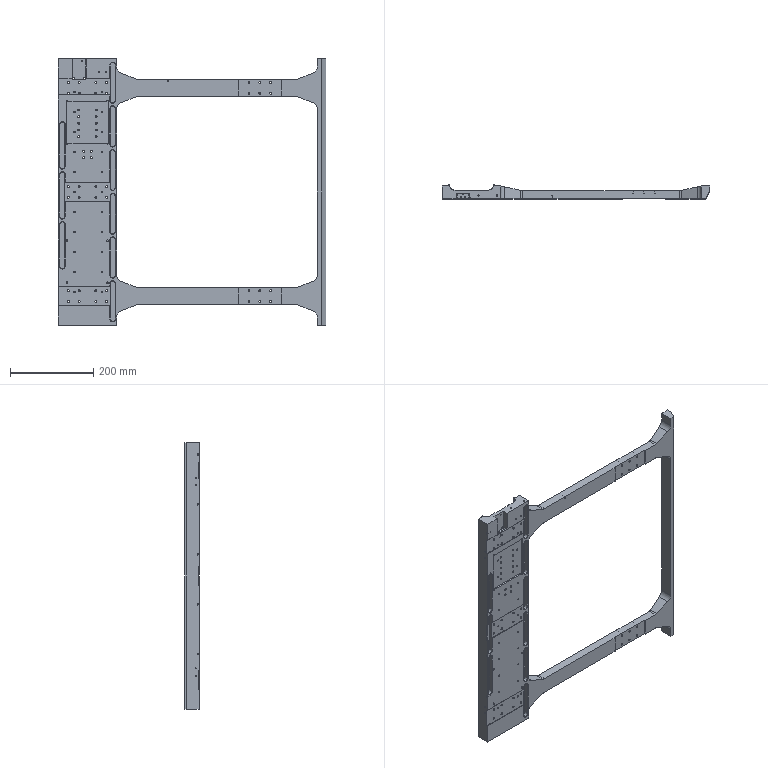Part | NX | features BREP 1 | 1 solid | 1056 faces | box 642 x 34 x 640 mm | volume 2797211 mm3 | cylinder 414 | plane 343 | cone 299 | commonest cylinder face diameters 3.3 x136 10 x112 4.5 x100 4 x20 30 x16 2.5 x10